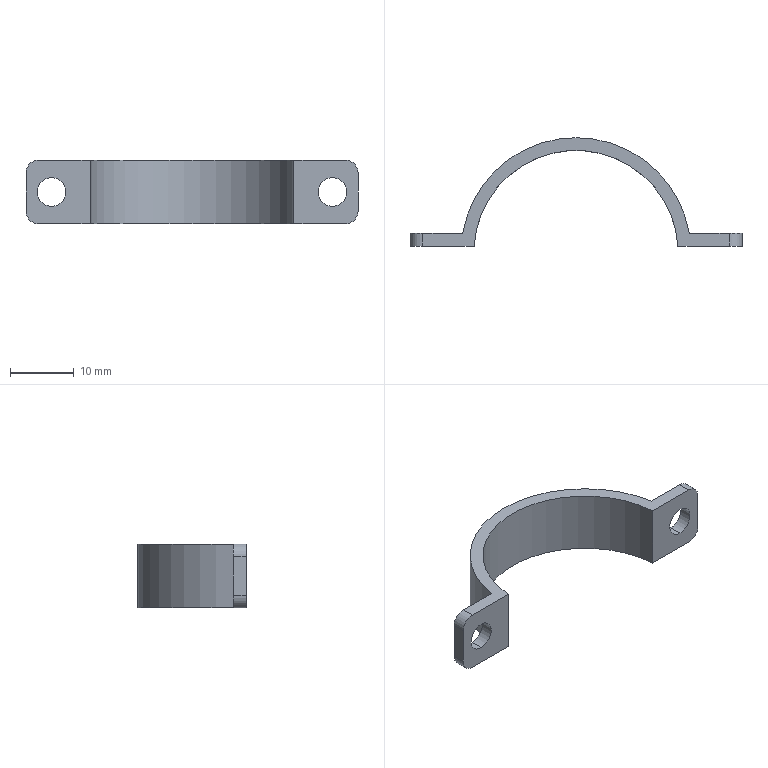Part | SolidWorks | features ExtruThin 1, Fillet 1, HoleWzd 1 | 1 solid | 18 faces | box 52 x 17 x 10 mm | volume 1282 mm3 | cylinder 10 | plane 8 | commonest cylinder face diameters 4 x4 4.5 x4 32 x1 36 x1
STEP:
#1=CARTESIAN_POINT('',(-6.031,0.,-2.75));
#2=VERTEX_POINT('',#1);
#3=CARTESIAN_POINT('',(-6.031,0.,-7.25));
#4=VERTEX_POINT('',#3);
#5=CARTESIAN_POINT('',(-6.031,0.,-5.));
#6=DIRECTION('',(0.,-1.,0.));
#7=DIRECTION('',(0.,0.,-1.));
#8=AXIS2_PLACEMENT_3D('',#5,#6,#7);
#9=CIRCLE('',#8,2.25);
#10=EDGE_CURVE('',#2,#4,#9,.T.);
#11=ORIENTED_EDGE('',*,*,#10,.T.);
#12=CARTESIAN_POINT('',(-6.031,2.,-7.25));
#13=VERTEX_POINT('',#12);
#14=CARTESIAN_POINT('',(-6.031,2.,-7.25));
#15=DIRECTION('',(0.,1.,0.));
#16=VECTOR('',#15,1000.);
#17=LINE('',#14,#16);
#18=EDGE_CURVE('',#4,#13,#17,.T.);
#19=ORIENTED_EDGE('',*,*,#18,.T.);
#20=CARTESIAN_POINT('',(-6.031,2.,-2.75));
#21=VERTEX_POINT('',#20);
#22=CARTESIAN_POINT('',(-6.031,2.,-5.));
#23=DIRECTION('',(0.,1.,0.));
#24=DIRECTION('',(0.,0.,1.));
#25=AXIS2_PLACEMENT_3D('',#22,#23,#24);
#26=CIRCLE('',#25,2.25);
#27=EDGE_CURVE('',#13,#21,#26,.T.);
#28=ORIENTED_EDGE('',*,*,#27,.T.);
#29=CARTESIAN_POINT('',(-6.031,2.,-2.75));
#30=DIRECTION('',(0.,1.,0.));
#31=VECTOR('',#30,1000.);
#32=LINE('',#29,#31);
#33=EDGE_CURVE('',#2,#21,#32,.T.);
#34=ORIENTED_EDGE('',*,*,#33,.F.);
#35=EDGE_LOOP('',(#11,#19,#28,#34));
#36=FACE_OUTER_BOUND('',#35,.T.);
#37=CARTESIAN_POINT('',(-6.031,2.,-5.));
#38=DIRECTION('',(0.,1.,0.));
#39=DIRECTION('',(0.,0.,1.));
#40=AXIS2_PLACEMENT_3D('',#37,#38,#39);
#41=CYLINDRICAL_SURFACE('',#40,2.25);
#42=ADVANCED_FACE('',(#36),#41,.F.);
#43=CARTESIAN_POINT('',(37.969,0.,-2.75));
#44=VERTEX_POINT('',#43);
#45=CARTESIAN_POINT('',(37.969,0.,-7.25));
#46=VERTEX_POINT('',#45);
#47=CARTESIAN_POINT('',(37.969,0.,-5.));
#48=DIRECTION('',(0.,-1.,0.));
#49=DIRECTION('',(0.,0.,-1.));
#50=AXIS2_PLACEMENT_3D('',#47,#48,#49);
#51=CIRCLE('',#50,2.25);
#52=EDGE_CURVE('',#44,#46,#51,.T.);
#53=ORIENTED_EDGE('',*,*,#52,.T.);
#54=CARTESIAN_POINT('',(37.969,2.,-7.25));
#55=VERTEX_POINT('',#54);
#56=CARTESIAN_POINT('',(37.969,2.,-7.25));
#57=DIRECTION('',(0.,1.,0.));
#58=VECTOR('',#57,1000.);
#59=LINE('',#56,#58);
#60=EDGE_CURVE('',#46,#55,#59,.T.);
#61=ORIENTED_EDGE('',*,*,#60,.T.);
#62=CARTESIAN_POINT('',(37.969,2.,-2.75));
#63=VERTEX_POINT('',#62);
#64=CARTESIAN_POINT('',(37.969,2.,-5.));
#65=DIRECTION('',(0.,1.,0.));
#66=DIRECTION('',(0.,0.,1.));
#67=AXIS2_PLACEMENT_3D('',#64,#65,#66);
#68=CIRCLE('',#67,2.25);
#69=EDGE_CURVE('',#55,#63,#68,.T.);
#70=ORIENTED_EDGE('',*,*,#69,.T.);
#71=CARTESIAN_POINT('',(37.969,2.,-2.75));
#72=DIRECTION('',(0.,1.,0.));
#73=VECTOR('',#72,1000.);
#74=LINE('',#71,#73);
#75=EDGE_CURVE('',#44,#63,#74,.T.);
#76=ORIENTED_EDGE('',*,*,#75,.F.);
#77=EDGE_LOOP('',(#53,#61,#70,#76));
#78=FACE_OUTER_BOUND('',#77,.T.);
#79=CARTESIAN_POINT('',(37.969,2.,-5.));
#80=DIRECTION('',(0.,1.,0.));
#81=DIRECTION('',(0.,0.,1.));
#82=AXIS2_PLACEMENT_3D('',#79,#80,#81);
#83=CYLINDRICAL_SURFACE('',#82,2.25);
#84=ADVANCED_FACE('',(#78),#83,.F.);
#85=ORIENTED_EDGE('',*,*,#52,.F.);
#86=CARTESIAN_POINT('',(37.969,0.,-5.));
#87=DIRECTION('',(0.,-1.,0.));
#88=DIRECTION('',(0.,0.,-1.));
#89=AXIS2_PLACEMENT_3D('',#86,#87,#88);
#90=CIRCLE('',#89,2.25);
#91=EDGE_CURVE('',#46,#44,#90,.T.);
#92=ORIENTED_EDGE('',*,*,#91,.F.);
#93=EDGE_LOOP('',(#85,#92));
#94=FACE_BOUND('',#93,.T.);
#95=CARTESIAN_POINT('',(31.937,0.,-10.));
#96=VERTEX_POINT('',#95);
#97=CARTESIAN_POINT('',(39.969,0.,-10.));
#98=VERTEX_POINT('',#97);
#99=CARTESIAN_POINT('',(31.937,0.,-10.));
#100=DIRECTION('',(1.,0.,0.));
#101=VECTOR('',#100,1000.);
#102=LINE('',#99,#101);
#103=EDGE_CURVE('',#96,#98,#102,.T.);
#104=ORIENTED_EDGE('',*,*,#103,.T.);
#105=CARTESIAN_POINT('',(41.969,0.,-8.));
#106=VERTEX_POINT('',#105);
#107=CARTESIAN_POINT('',(39.969,0.,-8.));
#108=DIRECTION('',(0.,-1.,0.));
#109=DIRECTION('',(0.,0.,-1.));
#110=AXIS2_PLACEMENT_3D('',#107,#108,#109);
#111=CIRCLE('',#110,2.);
#112=EDGE_CURVE('',#98,#106,#111,.T.);
#113=ORIENTED_EDGE('',*,*,#112,.T.);
#114=CARTESIAN_POINT('',(41.969,0.,-2.));
#115=VERTEX_POINT('',#114);
#116=CARTESIAN_POINT('',(41.969,0.,-10.));
#117=DIRECTION('',(0.,0.,1.));
#118=VECTOR('',#117,1000.);
#119=LINE('',#116,#118);
#120=EDGE_CURVE('',#106,#115,#119,.T.);
#121=ORIENTED_EDGE('',*,*,#120,.T.);
#122=CARTESIAN_POINT('',(39.969,0.,0.));
#123=VERTEX_POINT('',#122);
#124=CARTESIAN_POINT('',(39.969,0.,-2.));
#125=DIRECTION('',(0.,-1.,0.));
#126=DIRECTION('',(0.,0.,-1.));
#127=AXIS2_PLACEMENT_3D('',#124,#125,#126);
#128=CIRCLE('',#127,2.);
#129=EDGE_CURVE('',#115,#123,#128,.T.);
#130=ORIENTED_EDGE('',*,*,#129,.T.);
#131=CARTESIAN_POINT('',(31.937,0.,0.));
#132=VERTEX_POINT('',#131);
#133=CARTESIAN_POINT('',(31.937,0.,0.));
#134=DIRECTION('',(1.,0.,0.));
#135=VECTOR('',#134,1000.);
#136=LINE('',#133,#135);
#137=EDGE_CURVE('',#132,#123,#136,.T.);
#138=ORIENTED_EDGE('',*,*,#137,.F.);
#139=CARTESIAN_POINT('',(31.937,0.,-10.));
#140=DIRECTION('',(0.,0.,1.));
#141=VECTOR('',#140,1000.);
#142=LINE('',#139,#141);
#143=EDGE_CURVE('',#96,#132,#142,.T.);
#144=ORIENTED_EDGE('',*,*,#143,.F.);
#145=EDGE_LOOP('',(#104,#113,#121,#130,#138,#144));
#146=FACE_OUTER_BOUND('',#145,.T.);
#147=CARTESIAN_POINT('',(31.937,0.,-10.));
#148=DIRECTION('',(0.,-1.,0.));
#149=DIRECTION('',(0.,0.,-1.));
#150=AXIS2_PLACEMENT_3D('',#147,#148,#149);
#151=PLANE('',#150);
#152=ADVANCED_FACE('',(#94,#146),#151,.T.);
#153=CARTESIAN_POINT('',(0.,0.,0.));
#154=VERTEX_POINT('',#153);
#155=CARTESIAN_POINT('',(15.969,-1.,0.));
#156=DIRECTION('',(0.,0.,-1.));
#157=DIRECTION('',(-1.,0.,0.));
#158=AXIS2_PLACEMENT_3D('',#155,#156,#157);
#159=CIRCLE('',#158,16.);
#160=EDGE_CURVE('',#154,#132,#159,.T.);
#161=ORIENTED_EDGE('',*,*,#160,.F.);
#162=CARTESIAN_POINT('',(0.,0.,-10.));
#163=VERTEX_POINT('',#162);
#164=CARTESIAN_POINT('',(0.,0.,-10.));
#165=DIRECTION('',(0.,0.,1.));
#166=VECTOR('',#165,1000.);
#167=LINE('',#164,#166);
#168=EDGE_CURVE('',#163,#154,#167,.T.);
#169=ORIENTED_EDGE('',*,*,#168,.F.);
#170=CARTESIAN_POINT('',(15.969,-1.,-10.));
#171=DIRECTION('',(0.,0.,-1.));
#172=DIRECTION('',(-1.,0.,0.));
#173=AXIS2_PLACEMENT_3D('',#170,#171,#172);
#174=CIRCLE('',#173,16.);
#175=EDGE_CURVE('',#163,#96,#174,.T.);
#176=ORIENTED_EDGE('',*,*,#175,.T.);
#177=ORIENTED_EDGE('',*,*,#143,.T.);
#178=EDGE_LOOP('',(#161,#169,#176,#177));
#179=FACE_OUTER_BOUND('',#178,.T.);
#180=CARTESIAN_POINT('',(15.969,-1.,-10.));
#181=DIRECTION('',(0.,0.,1.));
#182=DIRECTION('',(1.,0.,0.));
#183=AXIS2_PLACEMENT_3D('',#180,#181,#182);
#184=CYLINDRICAL_SURFACE('',#183,16.);
#185=ADVANCED_FACE('',(#179),#184,.F.);
#186=ORIENTED_EDGE('',*,*,#10,.F.);
#187=CARTESIAN_POINT('',(-6.031,0.,-5.));
#188=DIRECTION('',(0.,-1.,0.));
#189=DIRECTION('',(0.,0.,-1.));
#190=AXIS2_PLACEMENT_3D('',#187,#188,#189);
#191=CIRCLE('',#190,2.25);
#192=EDGE_CURVE('',#4,#2,#191,.T.);
#193=ORIENTED_EDGE('',*,*,#192,.F.);
#194=EDGE_LOOP('',(#186,#193));
#195=FACE_BOUND('',#194,.T.);
#196=CARTESIAN_POINT('',(-8.031,0.,0.));
#197=VERTEX_POINT('',#196);
#198=CARTESIAN_POINT('',(0.,0.,0.));
#199=DIRECTION('',(1.,0.,0.));
#200=VECTOR('',#199,1000.);
#201=LINE('',#198,#200);
#202=EDGE_CURVE('',#197,#154,#201,.T.);
#203=ORIENTED_EDGE('',*,*,#202,.F.);
#204=CARTESIAN_POINT('',(-10.031,0.,-2.));
#205=VERTEX_POINT('',#204);
#206=CARTESIAN_POINT('',(-8.031,0.,-2.));
#207=DIRECTION('',(0.,-1.,0.));
#208=DIRECTION('',(0.,0.,-1.));
#209=AXIS2_PLACEMENT_3D('',#206,#207,#208);
#210=CIRCLE('',#209,2.);
#211=EDGE_CURVE('',#197,#205,#210,.T.);
#212=ORIENTED_EDGE('',*,*,#211,.T.);
#213=CARTESIAN_POINT('',(-10.031,0.,-8.));
#214=VERTEX_POINT('',#213);
#215=CARTESIAN_POINT('',(-10.031,0.,-10.));
#216=DIRECTION('',(0.,0.,1.));
#217=VECTOR('',#216,1000.);
#218=LINE('',#215,#217);
#219=EDGE_CURVE('',#214,#205,#218,.T.);
#220=ORIENTED_EDGE('',*,*,#219,.F.);
#221=CARTESIAN_POINT('',(-8.031,0.,-10.));
#222=VERTEX_POINT('',#221);
#223=CARTESIAN_POINT('',(-8.031,0.,-8.));
#224=DIRECTION('',(0.,-1.,0.));
#225=DIRECTION('',(0.,0.,-1.));
#226=AXIS2_PLACEMENT_3D('',#223,#224,#225);
#227=CIRCLE('',#226,2.);
#228=EDGE_CURVE('',#214,#222,#227,.T.);
#229=ORIENTED_EDGE('',*,*,#228,.T.);
#230=CARTESIAN_POINT('',(0.,0.,-10.));
#231=DIRECTION('',(1.,0.,0.));
#232=VECTOR('',#231,1000.);
#233=LINE('',#230,#232);
#234=EDGE_CURVE('',#222,#163,#233,.T.);
#235=ORIENTED_EDGE('',*,*,#234,.T.);
#236=ORIENTED_EDGE('',*,*,#168,.T.);
#237=EDGE_LOOP('',(#203,#212,#220,#229,#235,#236));
#238=FACE_OUTER_BOUND('',#237,.T.);
#239=CARTESIAN_POINT('',(0.,0.,-10.));
#240=DIRECTION('',(0.,-1.,0.));
#241=DIRECTION('',(0.,0.,-1.));
#242=AXIS2_PLACEMENT_3D('',#239,#240,#241);
#243=PLANE('',#242);
#244=ADVANCED_FACE('',(#195,#238),#243,.T.);
#245=ORIENTED_EDGE('',*,*,#219,.T.);
#246=CARTESIAN_POINT('',(-10.031,2.,-2.));
#247=VERTEX_POINT('',#246);
#248=CARTESIAN_POINT('',(-10.031,2.,-2.));
#249=DIRECTION('',(0.,1.,0.));
#250=VECTOR('',#249,1000.);
#251=LINE('',#248,#250);
#252=EDGE_CURVE('',#205,#247,#251,.T.);
#253=ORIENTED_EDGE('',*,*,#252,.T.);
#254=CARTESIAN_POINT('',(-10.031,2.,-8.));
#255=VERTEX_POINT('',#254);
#256=CARTESIAN_POINT('',(-10.031,2.,-10.));
#257=DIRECTION('',(0.,0.,1.));
#258=VECTOR('',#257,1000.);
#259=LINE('',#256,#258);
#260=EDGE_CURVE('',#255,#247,#259,.T.);
#261=ORIENTED_EDGE('',*,*,#260,.F.);
#262=CARTESIAN_POINT('',(-10.031,0.,-8.));
#263=DIRECTION('',(0.,-1.,0.));
#264=VECTOR('',#263,1000.);
#265=LINE('',#262,#264);
#266=EDGE_CURVE('',#255,#214,#265,.T.);
#267=ORIENTED_EDGE('',*,*,#266,.T.);
#268=EDGE_LOOP('',(#245,#253,#261,#267));
#269=FACE_OUTER_BOUND('',#268,.T.);
#270=CARTESIAN_POINT('',(-10.031,0.,-10.));
#271=DIRECTION('',(1.,0.,0.));
#272=DIRECTION('',(0.,0.,-1.));
#273=AXIS2_PLACEMENT_3D('',#270,#271,#272);
#274=PLANE('',#273);
#275=ADVANCED_FACE('',(#269),#274,.F.);
#276=CARTESIAN_POINT('',(-6.031,2.,-5.));
#277=DIRECTION('',(0.,1.,0.));
#278=DIRECTION('',(0.,0.,1.));
#279=AXIS2_PLACEMENT_3D('',#276,#277,#278);
#280=CIRCLE('',#279,2.25);
#281=EDGE_CURVE('',#21,#13,#280,.T.);
#282=ORIENTED_EDGE('',*,*,#281,.F.);
#283=ORIENTED_EDGE('',*,*,#27,.F.);
#284=EDGE_LOOP('',(#282,#283));
#285=FACE_BOUND('',#284,.T.);
#286=ORIENTED_EDGE('',*,*,#260,.T.);
#287=CARTESIAN_POINT('',(-8.031,2.,0.));
#288=VERTEX_POINT('',#287);
#289=CARTESIAN_POINT('',(-8.031,2.,-2.));
#290=DIRECTION('',(0.,1.,0.));
#291=DIRECTION('',(0.,0.,-1.));
#292=AXIS2_PLACEMENT_3D('',#289,#290,#291);
#293=CIRCLE('',#292,2.);
#294=EDGE_CURVE('',#247,#288,#293,.T.);
#295=ORIENTED_EDGE('',*,*,#294,.T.);
#296=CARTESIAN_POINT('',(-1.78,2.,0.));
#297=VERTEX_POINT('',#296);
#298=CARTESIAN_POINT('',(0.,2.,0.));
#299=DIRECTION('',(1.,0.,0.));
#300=VECTOR('',#299,1000.);
#301=LINE('',#298,#300);
#302=EDGE_CURVE('',#288,#297,#301,.T.);
#303=ORIENTED_EDGE('',*,*,#302,.T.);
#304=CARTESIAN_POINT('',(-1.78,2.,-10.));
#305=VERTEX_POINT('',#304);
#306=CARTESIAN_POINT('',(-1.78,2.,-10.));
#307=DIRECTION('',(0.,0.,1.));
#308=VECTOR('',#307,1000.);
#309=LINE('',#306,#308);
#310=EDGE_CURVE('',#305,#297,#309,.T.);
#311=ORIENTED_EDGE('',*,*,#310,.F.);
#312=CARTESIAN_POINT('',(-8.031,2.,-10.));
#313=VERTEX_POINT('',#312);
#314=CARTESIAN_POINT('',(0.,2.,-10.));
#315=DIRECTION('',(1.,0.,0.));
#316=VECTOR('',#315,1000.);
#317=LINE('',#314,#316);
#318=EDGE_CURVE('',#313,#305,#317,.T.);
#319=ORIENTED_EDGE('',*,*,#318,.F.);
#320=CARTESIAN_POINT('',(-8.031,2.,-8.));
#321=DIRECTION('',(0.,1.,0.));
#322=DIRECTION('',(0.,0.,-1.));
#323=AXIS2_PLACEMENT_3D('',#320,#321,#322);
#324=CIRCLE('',#323,2.);
#325=EDGE_CURVE('',#313,#255,#324,.T.);
#326=ORIENTED_EDGE('',*,*,#325,.T.);
#327=EDGE_LOOP('',(#286,#295,#303,#311,#319,#326));
#328=FACE_OUTER_BOUND('',#327,.T.);
#329=CARTESIAN_POINT('',(0.,2.,-10.));
#330=DIRECTION('',(0.,-1.,0.));
#331=DIRECTION('',(0.,0.,-1.));
#332=AXIS2_PLACEMENT_3D('',#329,#330,#331);
#333=PLANE('',#332);
#334=ADVANCED_FACE('',(#285,#328),#333,.F.);
#335=CARTESIAN_POINT('',(33.717,2.,0.));
#336=VERTEX_POINT('',#335);
#337=CARTESIAN_POINT('',(15.969,-1.,0.));
#338=DIRECTION('',(0.,0.,-1.));
#339=DIRECTION('',(1.,0.,0.));
#340=AXIS2_PLACEMENT_3D('',#337,#338,#339);
#341=CIRCLE('',#340,18.);
#342=EDGE_CURVE('',#297,#336,#341,.T.);
#343=ORIENTED_EDGE('',*,*,#342,.T.);
#344=CARTESIAN_POINT('',(33.717,2.,-10.));
#345=VERTEX_POINT('',#344);
#346=CARTESIAN_POINT('',(33.717,2.,-10.));
#347=DIRECTION('',(0.,0.,1.));
#348=VECTOR('',#347,1000.);
#349=LINE('',#346,#348);
#350=EDGE_CURVE('',#345,#336,#349,.T.);
#351=ORIENTED_EDGE('',*,*,#350,.F.);
#352=CARTESIAN_POINT('',(15.969,-1.,-10.));
#353=DIRECTION('',(0.,0.,-1.));
#354=DIRECTION('',(1.,0.,0.));
#355=AXIS2_PLACEMENT_3D('',#352,#353,#354);
#356=CIRCLE('',#355,18.);
#357=EDGE_CURVE('',#305,#345,#356,.T.);
#358=ORIENTED_EDGE('',*,*,#357,.F.);
#359=ORIENTED_EDGE('',*,*,#310,.T.);
#360=EDGE_LOOP('',(#343,#351,#358,#359));
#361=FACE_OUTER_BOUND('',#360,.T.);
#362=CARTESIAN_POINT('',(15.969,-1.,-10.));
#363=DIRECTION('',(0.,0.,1.));
#364=DIRECTION('',(1.,0.,0.));
#365=AXIS2_PLACEMENT_3D('',#362,#363,#364);
#366=CYLINDRICAL_SURFACE('',#365,18.);
#367=ADVANCED_FACE('',(#361),#366,.T.);
#368=CARTESIAN_POINT('',(37.969,2.,-5.));
#369=DIRECTION('',(0.,1.,0.));
#370=DIRECTION('',(0.,0.,1.));
#371=AXIS2_PLACEMENT_3D('',#368,#369,#370);
#372=CIRCLE('',#371,2.25);
#373=EDGE_CURVE('',#63,#55,#372,.T.);
#374=ORIENTED_EDGE('',*,*,#373,.F.);
#375=ORIENTED_EDGE('',*,*,#69,.F.);
#376=EDGE_LOOP('',(#374,#375));
#377=FACE_BOUND('',#376,.T.);
#378=CARTESIAN_POINT('',(41.969,2.,-8.));
#379=VERTEX_POINT('',#378);
#380=CARTESIAN_POINT('',(41.969,2.,-2.));
#381=VERTEX_POINT('',#380);
#382=CARTESIAN_POINT('',(41.969,2.,-10.));
#383=DIRECTION('',(0.,0.,1.));
#384=VECTOR('',#383,1000.);
#385=LINE('',#382,#384);
#386=EDGE_CURVE('',#379,#381,#385,.T.);
#387=ORIENTED_EDGE('',*,*,#386,.F.);
#388=CARTESIAN_POINT('',(39.969,2.,-10.));
#389=VERTEX_POINT('',#388);
#390=CARTESIAN_POINT('',(39.969,2.,-8.));
#391=DIRECTION('',(0.,1.,0.));
#392=DIRECTION('',(0.,0.,-1.));
#393=AXIS2_PLACEMENT_3D('',#390,#391,#392);
#394=CIRCLE('',#393,2.);
#395=EDGE_CURVE('',#379,#389,#394,.T.);
#396=ORIENTED_EDGE('',*,*,#395,.T.);
#397=CARTESIAN_POINT('',(31.937,2.,-10.));
#398=DIRECTION('',(1.,0.,0.));
#399=VECTOR('',#398,1000.);
#400=LINE('',#397,#399);
#401=EDGE_CURVE('',#345,#389,#400,.T.);
#402=ORIENTED_EDGE('',*,*,#401,.F.);
#403=ORIENTED_EDGE('',*,*,#350,.T.);
#404=CARTESIAN_POINT('',(39.969,2.,0.));
#405=VERTEX_POINT('',#404);
#406=CARTESIAN_POINT('',(31.937,2.,0.));
#407=DIRECTION('',(1.,0.,0.));
#408=VECTOR('',#407,1000.);
#409=LINE('',#406,#408);
#410=EDGE_CURVE('',#336,#405,#409,.T.);
#411=ORIENTED_EDGE('',*,*,#410,.T.);
#412=CARTESIAN_POINT('',(39.969,2.,-2.));
#413=DIRECTION('',(0.,1.,0.));
#414=DIRECTION('',(0.,0.,-1.));
#415=AXIS2_PLACEMENT_3D('',#412,#413,#414);
#416=CIRCLE('',#415,2.);
#417=EDGE_CURVE('',#405,#381,#416,.T.);
#418=ORIENTED_EDGE('',*,*,#417,.T.);
#419=EDGE_LOOP('',(#387,#396,#402,#403,#411,#418));
#420=FACE_OUTER_BOUND('',#419,.T.);
#421=CARTESIAN_POINT('',(31.937,2.,-10.));
#422=DIRECTION('',(0.,-1.,0.));
#423=DIRECTION('',(0.,0.,-1.));
#424=AXIS2_PLACEMENT_3D('',#421,#422,#423);
#425=PLANE('',#424);
#426=ADVANCED_FACE('',(#377,#420),#425,.F.);
#427=ORIENTED_EDGE('',*,*,#120,.F.);
#428=CARTESIAN_POINT('',(41.969,2.,-8.));
#429=DIRECTION('',(0.,1.,0.));
#430=VECTOR('',#429,1000.);
#431=LINE('',#428,#430);
#432=EDGE_CURVE('',#106,#379,#431,.T.);
#433=ORIENTED_EDGE('',*,*,#432,.T.);
#434=ORIENTED_EDGE('',*,*,#386,.T.);
#435=CARTESIAN_POINT('',(41.969,0.,-2.));
#436=DIRECTION('',(0.,-1.,0.));
#437=VECTOR('',#436,1000.);
#438=LINE('',#435,#437);
#439=EDGE_CURVE('',#381,#115,#438,.T.);
#440=ORIENTED_EDGE('',*,*,#439,.T.);
#441=EDGE_LOOP('',(#427,#433,#434,#440));
#442=FACE_OUTER_BOUND('',#441,.T.);
#443=CARTESIAN_POINT('',(41.969,2.,-10.));
#444=DIRECTION('',(-1.,0.,0.));
#445=DIRECTION('',(0.,0.,1.));
#446=AXIS2_PLACEMENT_3D('',#443,#444,#445);
#447=PLANE('',#446);
#448=ADVANCED_FACE('',(#442),#447,.F.);
#449=ORIENTED_EDGE('',*,*,#401,.T.);
#450=CARTESIAN_POINT('',(39.969,-1.,-10.));
#451=DIRECTION('',(0.,-1.,0.));
#452=VECTOR('',#451,1000.);
#453=LINE('',#450,#452);
#454=EDGE_CURVE('',#389,#98,#453,.T.);
#455=ORIENTED_EDGE('',*,*,#454,.T.);
#456=ORIENTED_EDGE('',*,*,#103,.F.);
#457=ORIENTED_EDGE('',*,*,#175,.F.);
#458=ORIENTED_EDGE('',*,*,#234,.F.);
#459=CARTESIAN_POINT('',(-8.031,-1.,-10.));
#460=DIRECTION('',(0.,1.,0.));
#461=VECTOR('',#460,1000.);
#462=LINE('',#459,#461);
#463=EDGE_CURVE('',#222,#313,#462,.T.);
#464=ORIENTED_EDGE('',*,*,#463,.T.);
#465=ORIENTED_EDGE('',*,*,#318,.T.);
#466=ORIENTED_EDGE('',*,*,#357,.T.);
#467=EDGE_LOOP('',(#449,#455,#456,#457,#458,#464,#465,#466));
#468=FACE_OUTER_BOUND('',#467,.T.);
#469=CARTESIAN_POINT('',(15.969,-1.,-10.));
#470=DIRECTION('',(0.,0.,1.));
#471=DIRECTION('',(1.,0.,0.));
#472=AXIS2_PLACEMENT_3D('',#469,#470,#471);
#473=PLANE('',#472);
#474=ADVANCED_FACE('',(#468),#473,.F.);
#475=ORIENTED_EDGE('',*,*,#137,.T.);
#476=CARTESIAN_POINT('',(39.969,2.,0.));
#477=DIRECTION('',(0.,1.,0.));
#478=VECTOR('',#477,1000.);
#479=LINE('',#476,#478);
#480=EDGE_CURVE('',#123,#405,#479,.T.);
#481=ORIENTED_EDGE('',*,*,#480,.T.);
#482=ORIENTED_EDGE('',*,*,#410,.F.);
#483=ORIENTED_EDGE('',*,*,#342,.F.);
#484=ORIENTED_EDGE('',*,*,#302,.F.);
#485=CARTESIAN_POINT('',(-8.031,0.,0.));
#486=DIRECTION('',(0.,-1.,0.));
#487=VECTOR('',#486,1000.);
#488=LINE('',#485,#487);
#489=EDGE_CURVE('',#288,#197,#488,.T.);
#490=ORIENTED_EDGE('',*,*,#489,.T.);
#491=ORIENTED_EDGE('',*,*,#202,.T.);
#492=ORIENTED_EDGE('',*,*,#160,.T.);
#493=EDGE_LOOP('',(#475,#481,#482,#483,#484,#490,#491,#492));
#494=FACE_OUTER_BOUND('',#493,.T.);
#495=CARTESIAN_POINT('',(15.969,-1.,0.));
#496=DIRECTION('',(0.,0.,1.));
#497=DIRECTION('',(1.,0.,0.));
#498=AXIS2_PLACEMENT_3D('',#495,#496,#497);
#499=PLANE('',#498);
#500=ADVANCED_FACE('',(#494),#499,.T.);
#501=ORIENTED_EDGE('',*,*,#60,.F.);
#502=ORIENTED_EDGE('',*,*,#91,.T.);
#503=ORIENTED_EDGE('',*,*,#75,.T.);
#504=ORIENTED_EDGE('',*,*,#373,.T.);
#505=EDGE_LOOP('',(#501,#502,#503,#504));
#506=FACE_OUTER_BOUND('',#505,.T.);
#507=CARTESIAN_POINT('',(37.969,2.,-5.));
#508=DIRECTION('',(0.,1.,0.));
#509=DIRECTION('',(0.,0.,1.));
#510=AXIS2_PLACEMENT_3D('',#507,#508,#509);
#511=CYLINDRICAL_SURFACE('',#510,2.25);
#512=ADVANCED_FACE('',(#506),#511,.F.);
#513=ORIENTED_EDGE('',*,*,#18,.F.);
#514=ORIENTED_EDGE('',*,*,#192,.T.);
#515=ORIENTED_EDGE('',*,*,#33,.T.);
#516=ORIENTED_EDGE('',*,*,#281,.T.);
#517=EDGE_LOOP('',(#513,#514,#515,#516));
#518=FACE_OUTER_BOUND('',#517,.T.);
#519=CARTESIAN_POINT('',(-6.031,2.,-5.));
#520=DIRECTION('',(0.,1.,0.));
#521=DIRECTION('',(0.,0.,1.));
#522=AXIS2_PLACEMENT_3D('',#519,#520,#521);
#523=CYLINDRICAL_SURFACE('',#522,2.25);
#524=ADVANCED_FACE('',(#518),#523,.F.);
#525=ORIENTED_EDGE('',*,*,#395,.F.);
#526=ORIENTED_EDGE('',*,*,#432,.F.);
#527=ORIENTED_EDGE('',*,*,#112,.F.);
#528=ORIENTED_EDGE('',*,*,#454,.F.);
#529=EDGE_LOOP('',(#525,#526,#527,#528));
#530=FACE_OUTER_BOUND('',#529,.T.);
#531=CARTESIAN_POINT('',(39.969,-1.,-8.));
#532=DIRECTION('',(0.,-1.,0.));
#533=DIRECTION('',(0.,0.,-1.));
#534=AXIS2_PLACEMENT_3D('',#531,#532,#533);
#535=CYLINDRICAL_SURFACE('',#534,2.);
#536=ADVANCED_FACE('',(#530),#535,.T.);
#537=ORIENTED_EDGE('',*,*,#417,.F.);
#538=ORIENTED_EDGE('',*,*,#480,.F.);
#539=ORIENTED_EDGE('',*,*,#129,.F.);
#540=ORIENTED_EDGE('',*,*,#439,.F.);
#541=EDGE_LOOP('',(#537,#538,#539,#540));
#542=FACE_OUTER_BOUND('',#541,.T.);
#543=CARTESIAN_POINT('',(39.969,2.,-2.));
#544=DIRECTION('',(0.,1.,0.));
#545=DIRECTION('',(0.,0.,1.));
#546=AXIS2_PLACEMENT_3D('',#543,#544,#545);
#547=CYLINDRICAL_SURFACE('',#546,2.);
#548=ADVANCED_FACE('',(#542),#547,.T.);
#549=ORIENTED_EDGE('',*,*,#211,.F.);
#550=ORIENTED_EDGE('',*,*,#489,.F.);
#551=ORIENTED_EDGE('',*,*,#294,.F.);
#552=ORIENTED_EDGE('',*,*,#252,.F.);
#553=EDGE_LOOP('',(#549,#550,#551,#552));
#554=FACE_OUTER_BOUND('',#553,.T.);
#555=CARTESIAN_POINT('',(-8.031,0.,-2.));
#556=DIRECTION('',(0.,-1.,0.));
#557=DIRECTION('',(0.,0.,-1.));
#558=AXIS2_PLACEMENT_3D('',#555,#556,#557);
#559=CYLINDRICAL_SURFACE('',#558,2.);
#560=ADVANCED_FACE('',(#554),#559,.T.);
#561=ORIENTED_EDGE('',*,*,#228,.F.);
#562=ORIENTED_EDGE('',*,*,#266,.F.);
#563=ORIENTED_EDGE('',*,*,#325,.F.);
#564=ORIENTED_EDGE('',*,*,#463,.F.);
#565=EDGE_LOOP('',(#561,#562,#563,#564));
#566=FACE_OUTER_BOUND('',#565,.T.);
#567=CARTESIAN_POINT('',(-8.031,-1.,-8.));
#568=DIRECTION('',(0.,1.,0.));
#569=DIRECTION('',(0.,0.,1.));
#570=AXIS2_PLACEMENT_3D('',#567,#568,#569);
#571=CYLINDRICAL_SURFACE('',#570,2.);
#572=ADVANCED_FACE('',(#566),#571,.T.);
#573=CLOSED_SHELL('',(#42,#84,#152,#185,#244,#275,#334,#367,#426,#448,#474,#500,#512,#524,#536,#548,#560,#572));
#574=MANIFOLD_SOLID_BREP('',#573);
#575=CARTESIAN_POINT('',(0.,0.,0.));
#576=DIRECTION('',(0.,0.,1.));
#577=DIRECTION('',(1.,0.,0.));
#578=AXIS2_PLACEMENT_3D('',#575,#576,#577);
#579=(LENGTH_UNIT()NAMED_UNIT(*)SI_UNIT(.MILLI.,.METRE.));
#580=UNCERTAINTY_MEASURE_WITH_UNIT(LENGTH_MEASURE(0.00001),#579,'','');
#581=(NAMED_UNIT(*)PLANE_ANGLE_UNIT()SI_UNIT($,.RADIAN.));
#582=(NAMED_UNIT(*)SI_UNIT($,.STERADIAN.)SOLID_ANGLE_UNIT());
#583=(GEOMETRIC_REPRESENTATION_CONTEXT(3)GLOBAL_UNCERTAINTY_ASSIGNED_CONTEXT((#580))GLOBAL_UNIT_ASSIGNED_CONTEXT((#579,#581,#582))REPRESENTATION_CONTEXT('',''));
#584=ADVANCED_BREP_SHAPE_REPRESENTATION('',(#574,#578),#583);